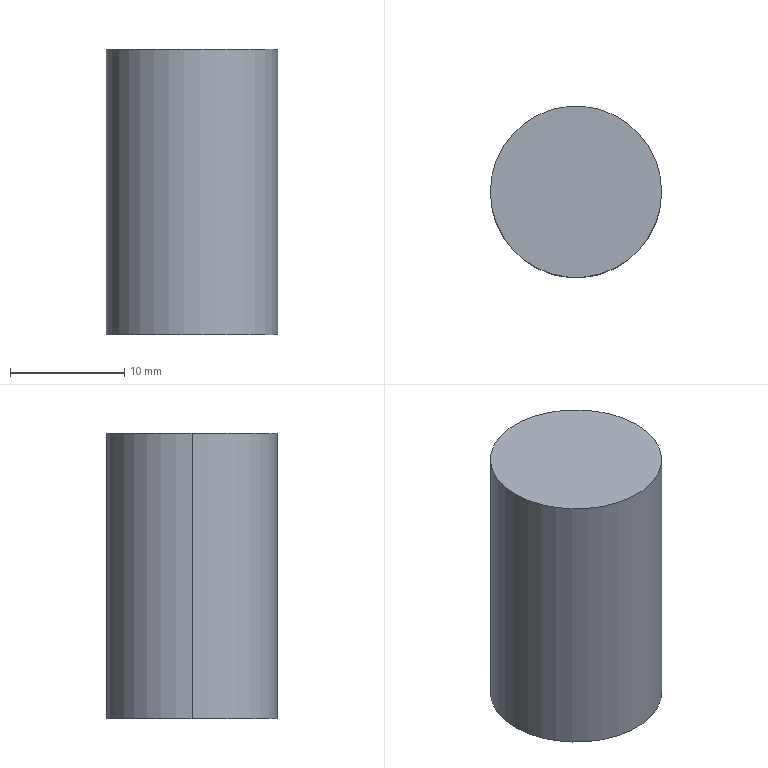Part | SolidWorks | features BaseBody 1 | 1 solid | 8 faces | box 15 x 15 x 25 mm | volume 4329 mm3 | cylinder 4 | cone 2 | plane 2 | commonest cylinder face diameters 3.3 x2 15 x2
STEP:
#1=CARTESIAN_POINT('',(1.65,0.,10.1));
#2=VERTEX_POINT('',#1);
#3=CARTESIAN_POINT('',(1.65,0.,0.));
#4=VERTEX_POINT('',#3);
#5=CARTESIAN_POINT('',(1.65,0.,0.));
#6=DIRECTION('',(0.,0.,-1.));
#7=VECTOR('',#6,1000.);
#8=LINE('',#5,#7);
#9=EDGE_CURVE('',#2,#4,#8,.T.);
#10=ORIENTED_EDGE('',*,*,#9,.F.);
#11=CARTESIAN_POINT('',(-1.65,0.,10.1));
#12=VERTEX_POINT('',#11);
#13=CARTESIAN_POINT('',(0.,0.,10.1));
#14=DIRECTION('',(0.,0.,-1.));
#15=DIRECTION('',(-1.,0.,0.));
#16=AXIS2_PLACEMENT_3D('',#13,#14,#15);
#17=CIRCLE('',#16,1.65);
#18=EDGE_CURVE('',#12,#2,#17,.T.);
#19=ORIENTED_EDGE('',*,*,#18,.F.);
#20=CARTESIAN_POINT('',(-1.65,0.,0.));
#21=VERTEX_POINT('',#20);
#22=CARTESIAN_POINT('',(-1.65,0.,0.));
#23=DIRECTION('',(0.,0.,-1.));
#24=VECTOR('',#23,1000.);
#25=LINE('',#22,#24);
#26=EDGE_CURVE('',#12,#21,#25,.T.);
#27=ORIENTED_EDGE('',*,*,#26,.T.);
#28=CARTESIAN_POINT('',(0.,0.,0.));
#29=DIRECTION('',(0.,0.,-1.));
#30=DIRECTION('',(-1.,0.,0.));
#31=AXIS2_PLACEMENT_3D('',#28,#29,#30);
#32=CIRCLE('',#31,1.65);
#33=EDGE_CURVE('',#21,#4,#32,.T.);
#34=ORIENTED_EDGE('',*,*,#33,.T.);
#35=EDGE_LOOP('',(#10,#19,#27,#34));
#36=FACE_OUTER_BOUND('',#35,.T.);
#37=CARTESIAN_POINT('',(0.,0.,0.));
#38=DIRECTION('',(0.,0.,-1.));
#39=DIRECTION('',(-1.,0.,0.));
#40=AXIS2_PLACEMENT_3D('',#37,#38,#39);
#41=CYLINDRICAL_SURFACE('',#40,1.65);
#42=ADVANCED_FACE('',(#36),#41,.F.);
#43=CARTESIAN_POINT('',(0.,0.,11.091));
#44=VERTEX_POINT('',#43);
#45=CARTESIAN_POINT('',(1.65,0.,10.1));
#46=DIRECTION('',(0.8572,0.,-0.515));
#47=VECTOR('',#46,1000.);
#48=LINE('',#45,#47);
#49=EDGE_CURVE('',#44,#2,#48,.T.);
#50=ORIENTED_EDGE('',*,*,#49,.F.);
#51=CARTESIAN_POINT('',(-1.65,0.,10.1));
#52=DIRECTION('',(-0.8572,0.,-0.515));
#53=VECTOR('',#52,1000.);
#54=LINE('',#51,#53);
#55=EDGE_CURVE('',#44,#12,#54,.T.);
#56=ORIENTED_EDGE('',*,*,#55,.T.);
#57=ORIENTED_EDGE('',*,*,#18,.T.);
#58=EDGE_LOOP('',(#50,#56,#57));
#59=FACE_OUTER_BOUND('',#58,.T.);
#60=CARTESIAN_POINT('',(0.,0.,10.1));
#61=DIRECTION('',(0.,0.,-1.));
#62=DIRECTION('',(-1.,0.,0.));
#63=AXIS2_PLACEMENT_3D('',#60,#61,#62);
#64=CONICAL_SURFACE('',#63,1.65,1.03);
#65=ADVANCED_FACE('',(#59),#64,.F.);
#66=ORIENTED_EDGE('',*,*,#33,.F.);
#67=CARTESIAN_POINT('',(0.,0.,0.));
#68=DIRECTION('',(0.,0.,-1.));
#69=DIRECTION('',(-1.,0.,0.));
#70=AXIS2_PLACEMENT_3D('',#67,#68,#69);
#71=CIRCLE('',#70,1.65);
#72=EDGE_CURVE('',#4,#21,#71,.T.);
#73=ORIENTED_EDGE('',*,*,#72,.F.);
#74=EDGE_LOOP('',(#66,#73));
#75=FACE_BOUND('',#74,.T.);
#76=CARTESIAN_POINT('',(-7.5,0.,0.));
#77=VERTEX_POINT('',#76);
#78=CARTESIAN_POINT('',(7.5,0.,0.));
#79=VERTEX_POINT('',#78);
#80=CARTESIAN_POINT('',(0.,0.,0.));
#81=DIRECTION('',(0.,0.,1.));
#82=DIRECTION('',(1.,0.,0.));
#83=AXIS2_PLACEMENT_3D('',#80,#81,#82);
#84=CIRCLE('',#83,7.5);
#85=EDGE_CURVE('',#77,#79,#84,.T.);
#86=ORIENTED_EDGE('',*,*,#85,.F.);
#87=CARTESIAN_POINT('',(0.,0.,0.));
#88=DIRECTION('',(0.,0.,1.));
#89=DIRECTION('',(1.,0.,0.));
#90=AXIS2_PLACEMENT_3D('',#87,#88,#89);
#91=CIRCLE('',#90,7.5);
#92=EDGE_CURVE('',#79,#77,#91,.T.);
#93=ORIENTED_EDGE('',*,*,#92,.F.);
#94=EDGE_LOOP('',(#86,#93));
#95=FACE_OUTER_BOUND('',#94,.T.);
#96=CARTESIAN_POINT('',(0.,0.,0.));
#97=DIRECTION('',(0.,0.,1.));
#98=DIRECTION('',(1.,0.,0.));
#99=AXIS2_PLACEMENT_3D('',#96,#97,#98);
#100=PLANE('',#99);
#101=ADVANCED_FACE('',(#75,#95),#100,.F.);
#102=CARTESIAN_POINT('',(-7.5,0.,25.));
#103=VERTEX_POINT('',#102);
#104=CARTESIAN_POINT('',(7.5,0.,25.));
#105=VERTEX_POINT('',#104);
#106=CARTESIAN_POINT('',(0.,0.,25.));
#107=DIRECTION('',(0.,0.,1.));
#108=DIRECTION('',(1.,0.,0.));
#109=AXIS2_PLACEMENT_3D('',#106,#107,#108);
#110=CIRCLE('',#109,7.5);
#111=EDGE_CURVE('',#103,#105,#110,.T.);
#112=ORIENTED_EDGE('',*,*,#111,.T.);
#113=CARTESIAN_POINT('',(0.,0.,25.));
#114=DIRECTION('',(0.,0.,1.));
#115=DIRECTION('',(1.,0.,0.));
#116=AXIS2_PLACEMENT_3D('',#113,#114,#115);
#117=CIRCLE('',#116,7.5);
#118=EDGE_CURVE('',#105,#103,#117,.T.);
#119=ORIENTED_EDGE('',*,*,#118,.T.);
#120=EDGE_LOOP('',(#112,#119));
#121=FACE_OUTER_BOUND('',#120,.T.);
#122=CARTESIAN_POINT('',(0.,0.,25.));
#123=DIRECTION('',(0.,0.,1.));
#124=DIRECTION('',(1.,0.,0.));
#125=AXIS2_PLACEMENT_3D('',#122,#123,#124);
#126=PLANE('',#125);
#127=ADVANCED_FACE('',(#121),#126,.T.);
#128=CARTESIAN_POINT('',(7.5,0.,25.));
#129=DIRECTION('',(0.,0.,-1.));
#130=VECTOR('',#129,1000.);
#131=LINE('',#128,#130);
#132=EDGE_CURVE('',#105,#79,#131,.T.);
#133=ORIENTED_EDGE('',*,*,#132,.F.);
#134=ORIENTED_EDGE('',*,*,#111,.F.);
#135=CARTESIAN_POINT('',(-7.5,0.,25.));
#136=DIRECTION('',(0.,0.,-1.));
#137=VECTOR('',#136,1000.);
#138=LINE('',#135,#137);
#139=EDGE_CURVE('',#103,#77,#138,.T.);
#140=ORIENTED_EDGE('',*,*,#139,.T.);
#141=ORIENTED_EDGE('',*,*,#85,.T.);
#142=EDGE_LOOP('',(#133,#134,#140,#141));
#143=FACE_OUTER_BOUND('',#142,.T.);
#144=CARTESIAN_POINT('',(0.,0.,25.));
#145=DIRECTION('',(0.,0.,-1.));
#146=DIRECTION('',(-1.,0.,0.));
#147=AXIS2_PLACEMENT_3D('',#144,#145,#146);
#148=CYLINDRICAL_SURFACE('',#147,7.5);
#149=ADVANCED_FACE('',(#143),#148,.T.);
#150=ORIENTED_EDGE('',*,*,#118,.F.);
#151=ORIENTED_EDGE('',*,*,#132,.T.);
#152=ORIENTED_EDGE('',*,*,#92,.T.);
#153=ORIENTED_EDGE('',*,*,#139,.F.);
#154=EDGE_LOOP('',(#150,#151,#152,#153));
#155=FACE_OUTER_BOUND('',#154,.T.);
#156=CARTESIAN_POINT('',(0.,0.,25.));
#157=DIRECTION('',(0.,0.,-1.));
#158=DIRECTION('',(-1.,0.,0.));
#159=AXIS2_PLACEMENT_3D('',#156,#157,#158);
#160=CYLINDRICAL_SURFACE('',#159,7.5);
#161=ADVANCED_FACE('',(#155),#160,.T.);
#162=ORIENTED_EDGE('',*,*,#55,.F.);
#163=ORIENTED_EDGE('',*,*,#49,.T.);
#164=CARTESIAN_POINT('',(0.,0.,10.1));
#165=DIRECTION('',(0.,0.,-1.));
#166=DIRECTION('',(-1.,0.,0.));
#167=AXIS2_PLACEMENT_3D('',#164,#165,#166);
#168=CIRCLE('',#167,1.65);
#169=EDGE_CURVE('',#2,#12,#168,.T.);
#170=ORIENTED_EDGE('',*,*,#169,.T.);
#171=EDGE_LOOP('',(#162,#163,#170));
#172=FACE_OUTER_BOUND('',#171,.T.);
#173=CARTESIAN_POINT('',(0.,0.,10.1));
#174=DIRECTION('',(0.,0.,-1.));
#175=DIRECTION('',(-1.,0.,0.));
#176=AXIS2_PLACEMENT_3D('',#173,#174,#175);
#177=CONICAL_SURFACE('',#176,1.65,1.03);
#178=ADVANCED_FACE('',(#172),#177,.F.);
#179=ORIENTED_EDGE('',*,*,#169,.F.);
#180=ORIENTED_EDGE('',*,*,#9,.T.);
#181=ORIENTED_EDGE('',*,*,#72,.T.);
#182=ORIENTED_EDGE('',*,*,#26,.F.);
#183=EDGE_LOOP('',(#179,#180,#181,#182));
#184=FACE_OUTER_BOUND('',#183,.T.);
#185=CARTESIAN_POINT('',(0.,0.,0.));
#186=DIRECTION('',(0.,0.,-1.));
#187=DIRECTION('',(-1.,0.,0.));
#188=AXIS2_PLACEMENT_3D('',#185,#186,#187);
#189=CYLINDRICAL_SURFACE('',#188,1.65);
#190=ADVANCED_FACE('',(#184),#189,.F.);
#191=CLOSED_SHELL('',(#42,#65,#101,#127,#149,#161,#178,#190));
#192=MANIFOLD_SOLID_BREP('',#191);
#193=CARTESIAN_POINT('',(0.,0.,0.));
#194=DIRECTION('',(0.,0.,1.));
#195=DIRECTION('',(1.,0.,0.));
#196=AXIS2_PLACEMENT_3D('',#193,#194,#195);
#197=(LENGTH_UNIT()NAMED_UNIT(*)SI_UNIT(.MILLI.,.METRE.));
#198=UNCERTAINTY_MEASURE_WITH_UNIT(LENGTH_MEASURE(0.00001),#197,'','');
#199=(NAMED_UNIT(*)PLANE_ANGLE_UNIT()SI_UNIT($,.RADIAN.));
#200=(NAMED_UNIT(*)SI_UNIT($,.STERADIAN.)SOLID_ANGLE_UNIT());
#201=(GEOMETRIC_REPRESENTATION_CONTEXT(3)GLOBAL_UNCERTAINTY_ASSIGNED_CONTEXT((#198))GLOBAL_UNIT_ASSIGNED_CONTEXT((#197,#199,#200))REPRESENTATION_CONTEXT('',''));
#202=ADVANCED_BREP_SHAPE_REPRESENTATION('',(#192,#196),#201);